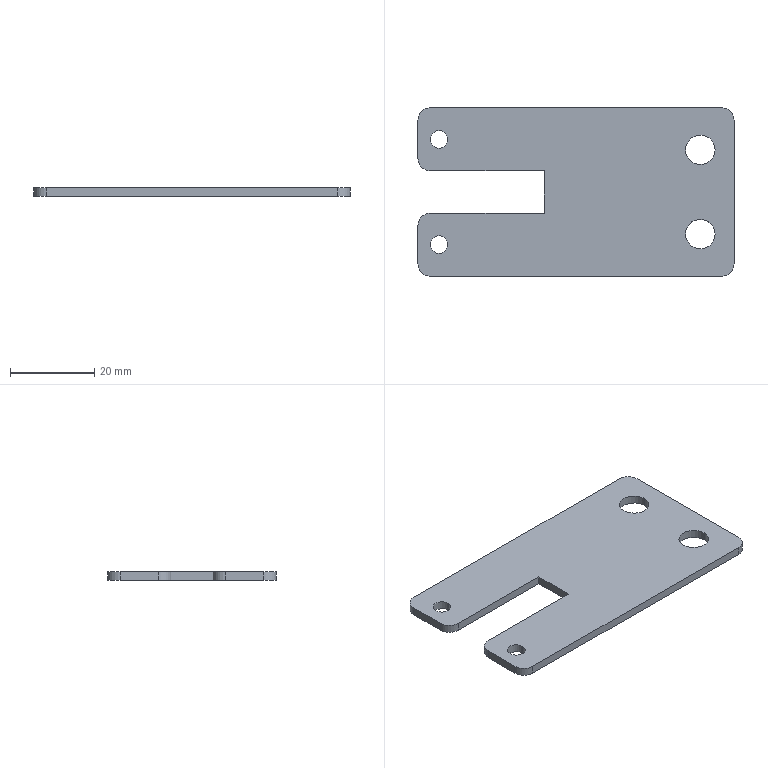Part | STEP file | 1 solid | 24 faces | box 75 x 40 x 2 mm | volume 5167 mm3 | cylinder 14 | plane 10 | commonest cylinder face diameters 6 x6 4.2 x4 7 x4